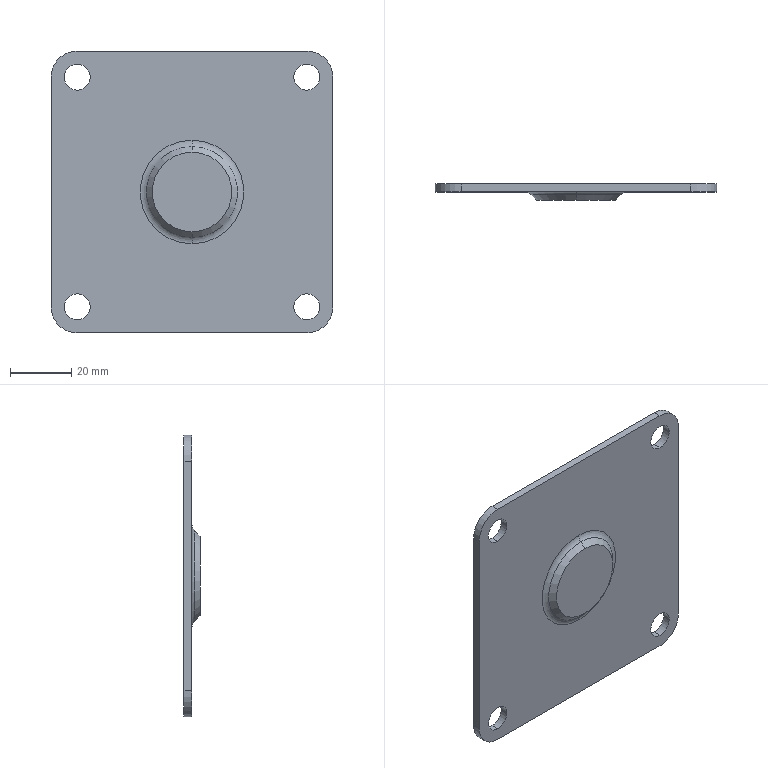Part | SolidWorks | features BaseBody 1 | 1 solid | 37 faces | box 92 x 5.3 x 92 mm | volume 22833 mm3 | cylinder 16 | torus 10 | plane 9 | cone 2 | commonest cylinder face diameters 8.5 x8 17 x6 20 x2
STEP:
#1=CARTESIAN_POINT('',(0.,0.,-13.));
#2=VERTEX_POINT('',#1);
#3=CARTESIAN_POINT('',(0.,0.,13.));
#4=VERTEX_POINT('',#3);
#5=CARTESIAN_POINT('',(0.,0.,0.));
#6=DIRECTION('',(0.,-1.,0.));
#7=DIRECTION('',(0.,0.,-1.));
#8=AXIS2_PLACEMENT_3D('',#5,#6,#7);
#9=CIRCLE('',#8,13.);
#10=EDGE_CURVE('',#2,#4,#9,.T.);
#11=ORIENTED_EDGE('',*,*,#10,.F.);
#12=CARTESIAN_POINT('',(0.,1.821,-14.821));
#13=VERTEX_POINT('',#12);
#14=CARTESIAN_POINT('',(0.,1.821,-14.821));
#15=DIRECTION('',(0.,0.7071,-0.7071));
#16=VECTOR('',#15,1000.);
#17=LINE('',#14,#16);
#18=EDGE_CURVE('',#2,#13,#17,.T.);
#19=ORIENTED_EDGE('',*,*,#18,.T.);
#20=CARTESIAN_POINT('',(0.,1.821,14.821));
#21=VERTEX_POINT('',#20);
#22=CARTESIAN_POINT('',(0.,1.821,0.));
#23=DIRECTION('',(0.,-1.,0.));
#24=DIRECTION('',(0.,0.,-1.));
#25=AXIS2_PLACEMENT_3D('',#22,#23,#24);
#26=CIRCLE('',#25,14.821);
#27=EDGE_CURVE('',#13,#21,#26,.T.);
#28=ORIENTED_EDGE('',*,*,#27,.T.);
#29=CARTESIAN_POINT('',(0.,1.821,14.821));
#30=DIRECTION('',(0.,0.7071,0.7071));
#31=VECTOR('',#30,1000.);
#32=LINE('',#29,#31);
#33=EDGE_CURVE('',#4,#21,#32,.T.);
#34=ORIENTED_EDGE('',*,*,#33,.F.);
#35=EDGE_LOOP('',(#11,#19,#28,#34));
#36=FACE_OUTER_BOUND('',#35,.T.);
#37=CARTESIAN_POINT('',(0.,1.821,0.));
#38=DIRECTION('',(0.,1.,0.));
#39=DIRECTION('',(0.,0.,1.));
#40=AXIS2_PLACEMENT_3D('',#37,#38,#39);
#41=CONICAL_SURFACE('',#40,14.821,0.7854);
#42=ADVANCED_FACE('',(#36),#41,.T.);
#43=CARTESIAN_POINT('',(0.,1.821,0.));
#44=DIRECTION('',(0.,-1.,0.));
#45=DIRECTION('',(0.,0.,-1.));
#46=AXIS2_PLACEMENT_3D('',#43,#44,#45);
#47=CIRCLE('',#46,14.821);
#48=EDGE_CURVE('',#21,#13,#47,.T.);
#49=ORIENTED_EDGE('',*,*,#48,.F.);
#50=CARTESIAN_POINT('',(0.,2.7,16.943));
#51=VERTEX_POINT('',#50);
#52=CARTESIAN_POINT('',(0.,-0.3,16.943));
#53=DIRECTION('',(1.,0.,0.));
#54=DIRECTION('',(0.,0.,-1.));
#55=AXIS2_PLACEMENT_3D('',#52,#53,#54);
#56=CIRCLE('',#55,3.);
#57=EDGE_CURVE('',#21,#51,#56,.T.);
#58=ORIENTED_EDGE('',*,*,#57,.T.);
#59=CARTESIAN_POINT('',(0.,2.7,-16.943));
#60=VERTEX_POINT('',#59);
#61=CARTESIAN_POINT('',(0.,2.7,0.));
#62=DIRECTION('',(0.,-1.,0.));
#63=DIRECTION('',(0.,0.,-1.));
#64=AXIS2_PLACEMENT_3D('',#61,#62,#63);
#65=CIRCLE('',#64,16.943);
#66=EDGE_CURVE('',#51,#60,#65,.T.);
#67=ORIENTED_EDGE('',*,*,#66,.T.);
#68=CARTESIAN_POINT('',(0.,-0.3,-16.943));
#69=DIRECTION('',(-1.,0.,0.));
#70=DIRECTION('',(0.,0.,1.));
#71=AXIS2_PLACEMENT_3D('',#68,#69,#70);
#72=CIRCLE('',#71,3.);
#73=EDGE_CURVE('',#13,#60,#72,.T.);
#74=ORIENTED_EDGE('',*,*,#73,.F.);
#75=EDGE_LOOP('',(#49,#58,#67,#74));
#76=FACE_OUTER_BOUND('',#75,.T.);
#77=CARTESIAN_POINT('',(0.,-0.3,0.));
#78=DIRECTION('',(0.,-1.,0.));
#79=DIRECTION('',(0.,0.,-1.));
#80=AXIS2_PLACEMENT_3D('',#77,#78,#79);
#81=TOROIDAL_SURFACE('',#80,16.943,3.);
#82=ADVANCED_FACE('',(#76),#81,.F.);
#83=CARTESIAN_POINT('',(-37.5,5.3,-41.75));
#84=VERTEX_POINT('',#83);
#85=CARTESIAN_POINT('',(-37.5,5.3,-33.25));
#86=VERTEX_POINT('',#85);
#87=CARTESIAN_POINT('',(-37.5,5.3,-37.5));
#88=DIRECTION('',(0.,1.,0.));
#89=DIRECTION('',(0.,0.,-1.));
#90=AXIS2_PLACEMENT_3D('',#87,#88,#89);
#91=CIRCLE('',#90,4.25);
#92=EDGE_CURVE('',#84,#86,#91,.T.);
#93=ORIENTED_EDGE('',*,*,#92,.T.);
#94=CARTESIAN_POINT('',(-37.5,2.7,-33.25));
#95=VERTEX_POINT('',#94);
#96=CARTESIAN_POINT('',(-37.5,5.6,-33.25));
#97=DIRECTION('',(0.,-1.,0.));
#98=VECTOR('',#97,1000.);
#99=LINE('',#96,#98);
#100=EDGE_CURVE('',#86,#95,#99,.T.);
#101=ORIENTED_EDGE('',*,*,#100,.T.);
#102=CARTESIAN_POINT('',(-37.5,2.7,-41.75));
#103=VERTEX_POINT('',#102);
#104=CARTESIAN_POINT('',(-37.5,2.7,-37.5));
#105=DIRECTION('',(0.,-1.,0.));
#106=DIRECTION('',(0.,0.,1.));
#107=AXIS2_PLACEMENT_3D('',#104,#105,#106);
#108=CIRCLE('',#107,4.25);
#109=EDGE_CURVE('',#95,#103,#108,.T.);
#110=ORIENTED_EDGE('',*,*,#109,.T.);
#111=CARTESIAN_POINT('',(-37.5,5.6,-41.75));
#112=DIRECTION('',(0.,-1.,0.));
#113=VECTOR('',#112,1000.);
#114=LINE('',#111,#113);
#115=EDGE_CURVE('',#84,#103,#114,.T.);
#116=ORIENTED_EDGE('',*,*,#115,.F.);
#117=EDGE_LOOP('',(#93,#101,#110,#116));
#118=FACE_OUTER_BOUND('',#117,.T.);
#119=CARTESIAN_POINT('',(-37.5,5.6,-37.5));
#120=DIRECTION('',(0.,-1.,0.));
#121=DIRECTION('',(0.,0.,-1.));
#122=AXIS2_PLACEMENT_3D('',#119,#120,#121);
#123=CYLINDRICAL_SURFACE('',#122,4.25);
#124=ADVANCED_FACE('',(#118),#123,.F.);
#125=CARTESIAN_POINT('',(-37.5,5.3,33.25));
#126=VERTEX_POINT('',#125);
#127=CARTESIAN_POINT('',(-37.5,5.3,41.75));
#128=VERTEX_POINT('',#127);
#129=CARTESIAN_POINT('',(-37.5,5.3,37.5));
#130=DIRECTION('',(0.,1.,0.));
#131=DIRECTION('',(0.,0.,-1.));
#132=AXIS2_PLACEMENT_3D('',#129,#130,#131);
#133=CIRCLE('',#132,4.25);
#134=EDGE_CURVE('',#126,#128,#133,.T.);
#135=ORIENTED_EDGE('',*,*,#134,.T.);
#136=CARTESIAN_POINT('',(-37.5,2.7,41.75));
#137=VERTEX_POINT('',#136);
#138=CARTESIAN_POINT('',(-37.5,5.6,41.75));
#139=DIRECTION('',(0.,-1.,0.));
#140=VECTOR('',#139,1000.);
#141=LINE('',#138,#140);
#142=EDGE_CURVE('',#128,#137,#141,.T.);
#143=ORIENTED_EDGE('',*,*,#142,.T.);
#144=CARTESIAN_POINT('',(-37.5,2.7,33.25));
#145=VERTEX_POINT('',#144);
#146=CARTESIAN_POINT('',(-37.5,2.7,37.5));
#147=DIRECTION('',(0.,-1.,0.));
#148=DIRECTION('',(0.,0.,1.));
#149=AXIS2_PLACEMENT_3D('',#146,#147,#148);
#150=CIRCLE('',#149,4.25);
#151=EDGE_CURVE('',#137,#145,#150,.T.);
#152=ORIENTED_EDGE('',*,*,#151,.T.);
#153=CARTESIAN_POINT('',(-37.5,5.6,33.25));
#154=DIRECTION('',(0.,-1.,0.));
#155=VECTOR('',#154,1000.);
#156=LINE('',#153,#155);
#157=EDGE_CURVE('',#126,#145,#156,.T.);
#158=ORIENTED_EDGE('',*,*,#157,.F.);
#159=EDGE_LOOP('',(#135,#143,#152,#158));
#160=FACE_OUTER_BOUND('',#159,.T.);
#161=CARTESIAN_POINT('',(-37.5,5.6,37.5));
#162=DIRECTION('',(0.,-1.,0.));
#163=DIRECTION('',(0.,0.,-1.));
#164=AXIS2_PLACEMENT_3D('',#161,#162,#163);
#165=CYLINDRICAL_SURFACE('',#164,4.25);
#166=ADVANCED_FACE('',(#160),#165,.F.);
#167=CARTESIAN_POINT('',(37.5,5.3,33.25));
#168=VERTEX_POINT('',#167);
#169=CARTESIAN_POINT('',(37.5,5.3,41.75));
#170=VERTEX_POINT('',#169);
#171=CARTESIAN_POINT('',(37.5,5.3,37.5));
#172=DIRECTION('',(0.,1.,0.));
#173=DIRECTION('',(0.,0.,-1.));
#174=AXIS2_PLACEMENT_3D('',#171,#172,#173);
#175=CIRCLE('',#174,4.25);
#176=EDGE_CURVE('',#168,#170,#175,.T.);
#177=ORIENTED_EDGE('',*,*,#176,.T.);
#178=CARTESIAN_POINT('',(37.5,2.7,41.75));
#179=VERTEX_POINT('',#178);
#180=CARTESIAN_POINT('',(37.5,5.6,41.75));
#181=DIRECTION('',(0.,-1.,0.));
#182=VECTOR('',#181,1000.);
#183=LINE('',#180,#182);
#184=EDGE_CURVE('',#170,#179,#183,.T.);
#185=ORIENTED_EDGE('',*,*,#184,.T.);
#186=CARTESIAN_POINT('',(37.5,2.7,33.25));
#187=VERTEX_POINT('',#186);
#188=CARTESIAN_POINT('',(37.5,2.7,37.5));
#189=DIRECTION('',(0.,-1.,0.));
#190=DIRECTION('',(0.,0.,1.));
#191=AXIS2_PLACEMENT_3D('',#188,#189,#190);
#192=CIRCLE('',#191,4.25);
#193=EDGE_CURVE('',#179,#187,#192,.T.);
#194=ORIENTED_EDGE('',*,*,#193,.T.);
#195=CARTESIAN_POINT('',(37.5,5.6,33.25));
#196=DIRECTION('',(0.,-1.,0.));
#197=VECTOR('',#196,1000.);
#198=LINE('',#195,#197);
#199=EDGE_CURVE('',#168,#187,#198,.T.);
#200=ORIENTED_EDGE('',*,*,#199,.F.);
#201=EDGE_LOOP('',(#177,#185,#194,#200));
#202=FACE_OUTER_BOUND('',#201,.T.);
#203=CARTESIAN_POINT('',(37.5,5.6,37.5));
#204=DIRECTION('',(0.,-1.,0.));
#205=DIRECTION('',(0.,0.,-1.));
#206=AXIS2_PLACEMENT_3D('',#203,#204,#205);
#207=CYLINDRICAL_SURFACE('',#206,4.25);
#208=ADVANCED_FACE('',(#202),#207,.F.);
#209=CARTESIAN_POINT('',(37.5,5.3,-41.75));
#210=VERTEX_POINT('',#209);
#211=CARTESIAN_POINT('',(37.5,5.3,-33.25));
#212=VERTEX_POINT('',#211);
#213=CARTESIAN_POINT('',(37.5,5.3,-37.5));
#214=DIRECTION('',(0.,1.,0.));
#215=DIRECTION('',(0.,0.,-1.));
#216=AXIS2_PLACEMENT_3D('',#213,#214,#215);
#217=CIRCLE('',#216,4.25);
#218=EDGE_CURVE('',#210,#212,#217,.T.);
#219=ORIENTED_EDGE('',*,*,#218,.T.);
#220=CARTESIAN_POINT('',(37.5,2.7,-33.25));
#221=VERTEX_POINT('',#220);
#222=CARTESIAN_POINT('',(37.5,5.6,-33.25));
#223=DIRECTION('',(0.,-1.,0.));
#224=VECTOR('',#223,1000.);
#225=LINE('',#222,#224);
#226=EDGE_CURVE('',#212,#221,#225,.T.);
#227=ORIENTED_EDGE('',*,*,#226,.T.);
#228=CARTESIAN_POINT('',(37.5,2.7,-41.75));
#229=VERTEX_POINT('',#228);
#230=CARTESIAN_POINT('',(37.5,2.7,-37.5));
#231=DIRECTION('',(0.,-1.,0.));
#232=DIRECTION('',(0.,0.,1.));
#233=AXIS2_PLACEMENT_3D('',#230,#231,#232);
#234=CIRCLE('',#233,4.25);
#235=EDGE_CURVE('',#221,#229,#234,.T.);
#236=ORIENTED_EDGE('',*,*,#235,.T.);
#237=CARTESIAN_POINT('',(37.5,5.6,-41.75));
#238=DIRECTION('',(0.,-1.,0.));
#239=VECTOR('',#238,1000.);
#240=LINE('',#237,#239);
#241=EDGE_CURVE('',#210,#229,#240,.T.);
#242=ORIENTED_EDGE('',*,*,#241,.F.);
#243=EDGE_LOOP('',(#219,#227,#236,#242));
#244=FACE_OUTER_BOUND('',#243,.T.);
#245=CARTESIAN_POINT('',(37.5,5.6,-37.5));
#246=DIRECTION('',(0.,-1.,0.));
#247=DIRECTION('',(0.,0.,-1.));
#248=AXIS2_PLACEMENT_3D('',#245,#246,#247);
#249=CYLINDRICAL_SURFACE('',#248,4.25);
#250=ADVANCED_FACE('',(#244),#249,.F.);
#251=CARTESIAN_POINT('',(0.,4.3,-10.));
#252=VERTEX_POINT('',#251);
#253=CARTESIAN_POINT('',(0.,4.3,10.));
#254=VERTEX_POINT('',#253);
#255=CARTESIAN_POINT('',(0.,4.3,0.));
#256=DIRECTION('',(0.,-1.,0.));
#257=DIRECTION('',(0.,0.,-1.));
#258=AXIS2_PLACEMENT_3D('',#255,#256,#257);
#259=CIRCLE('',#258,10.);
#260=EDGE_CURVE('',#252,#254,#259,.T.);
#261=ORIENTED_EDGE('',*,*,#260,.T.);
#262=CARTESIAN_POINT('',(0.,5.3,11.));
#263=VERTEX_POINT('',#262);
#264=CARTESIAN_POINT('',(0.,4.3,11.));
#265=DIRECTION('',(1.,0.,0.));
#266=DIRECTION('',(0.,0.,-1.));
#267=AXIS2_PLACEMENT_3D('',#264,#265,#266);
#268=CIRCLE('',#267,1.);
#269=EDGE_CURVE('',#254,#263,#268,.T.);
#270=ORIENTED_EDGE('',*,*,#269,.T.);
#271=CARTESIAN_POINT('',(0.,5.3,-11.));
#272=VERTEX_POINT('',#271);
#273=CARTESIAN_POINT('',(0.,5.3,0.));
#274=DIRECTION('',(0.,-1.,0.));
#275=DIRECTION('',(0.,0.,-1.));
#276=AXIS2_PLACEMENT_3D('',#273,#274,#275);
#277=CIRCLE('',#276,11.);
#278=EDGE_CURVE('',#272,#263,#277,.T.);
#279=ORIENTED_EDGE('',*,*,#278,.F.);
#280=CARTESIAN_POINT('',(0.,4.3,-11.));
#281=DIRECTION('',(-1.,0.,0.));
#282=DIRECTION('',(0.,0.,1.));
#283=AXIS2_PLACEMENT_3D('',#280,#281,#282);
#284=CIRCLE('',#283,1.);
#285=EDGE_CURVE('',#252,#272,#284,.T.);
#286=ORIENTED_EDGE('',*,*,#285,.F.);
#287=EDGE_LOOP('',(#261,#270,#279,#286));
#288=FACE_OUTER_BOUND('',#287,.T.);
#289=CARTESIAN_POINT('',(0.,4.3,0.));
#290=DIRECTION('',(0.,-1.,0.));
#291=DIRECTION('',(0.,0.,-1.));
#292=AXIS2_PLACEMENT_3D('',#289,#290,#291);
#293=TOROIDAL_SURFACE('',#292,11.,1.);
#294=ADVANCED_FACE('',(#288),#293,.T.);
#295=CARTESIAN_POINT('',(0.,4.3,0.));
#296=DIRECTION('',(0.,-1.,0.));
#297=DIRECTION('',(0.,0.,-1.));
#298=AXIS2_PLACEMENT_3D('',#295,#296,#297);
#299=CIRCLE('',#298,10.);
#300=EDGE_CURVE('',#254,#252,#299,.T.);
#301=ORIENTED_EDGE('',*,*,#300,.F.);
#302=CARTESIAN_POINT('',(0.,3.8,10.));
#303=VERTEX_POINT('',#302);
#304=CARTESIAN_POINT('',(0.,0.,10.));
#305=DIRECTION('',(0.,-1.,0.));
#306=VECTOR('',#305,1000.);
#307=LINE('',#304,#306);
#308=EDGE_CURVE('',#254,#303,#307,.T.);
#309=ORIENTED_EDGE('',*,*,#308,.T.);
#310=CARTESIAN_POINT('',(0.,3.8,-10.));
#311=VERTEX_POINT('',#310);
#312=CARTESIAN_POINT('',(0.,3.8,0.));
#313=DIRECTION('',(0.,-1.,0.));
#314=DIRECTION('',(0.,0.,-1.));
#315=AXIS2_PLACEMENT_3D('',#312,#313,#314);
#316=CIRCLE('',#315,10.);
#317=EDGE_CURVE('',#303,#311,#316,.T.);
#318=ORIENTED_EDGE('',*,*,#317,.T.);
#319=CARTESIAN_POINT('',(0.,0.,-10.));
#320=DIRECTION('',(0.,-1.,0.));
#321=VECTOR('',#320,1000.);
#322=LINE('',#319,#321);
#323=EDGE_CURVE('',#252,#311,#322,.T.);
#324=ORIENTED_EDGE('',*,*,#323,.F.);
#325=EDGE_LOOP('',(#301,#309,#318,#324));
#326=FACE_OUTER_BOUND('',#325,.T.);
#327=CARTESIAN_POINT('',(0.,0.,0.));
#328=DIRECTION('',(0.,-1.,0.));
#329=DIRECTION('',(0.,0.,-1.));
#330=AXIS2_PLACEMENT_3D('',#327,#328,#329);
#331=CYLINDRICAL_SURFACE('',#330,10.);
#332=ADVANCED_FACE('',(#326),#331,.F.);
#333=ORIENTED_EDGE('',*,*,#317,.F.);
#334=CARTESIAN_POINT('',(0.,3.3,9.5));
#335=VERTEX_POINT('',#334);
#336=CARTESIAN_POINT('',(0.,3.8,9.5));
#337=DIRECTION('',(1.,0.,0.));
#338=DIRECTION('',(0.,0.,-1.));
#339=AXIS2_PLACEMENT_3D('',#336,#337,#338);
#340=CIRCLE('',#339,0.5);
#341=EDGE_CURVE('',#303,#335,#340,.T.);
#342=ORIENTED_EDGE('',*,*,#341,.T.);
#343=CARTESIAN_POINT('',(0.,3.3,-9.5));
#344=VERTEX_POINT('',#343);
#345=CARTESIAN_POINT('',(0.,3.3,0.));
#346=DIRECTION('',(0.,-1.,0.));
#347=DIRECTION('',(0.,0.,-1.));
#348=AXIS2_PLACEMENT_3D('',#345,#346,#347);
#349=CIRCLE('',#348,9.5);
#350=EDGE_CURVE('',#335,#344,#349,.T.);
#351=ORIENTED_EDGE('',*,*,#350,.T.);
#352=CARTESIAN_POINT('',(0.,3.8,-9.5));
#353=DIRECTION('',(-1.,0.,0.));
#354=DIRECTION('',(0.,0.,1.));
#355=AXIS2_PLACEMENT_3D('',#352,#353,#354);
#356=CIRCLE('',#355,0.5);
#357=EDGE_CURVE('',#311,#344,#356,.T.);
#358=ORIENTED_EDGE('',*,*,#357,.F.);
#359=EDGE_LOOP('',(#333,#342,#351,#358));
#360=FACE_OUTER_BOUND('',#359,.T.);
#361=CARTESIAN_POINT('',(0.,3.8,0.));
#362=DIRECTION('',(0.,-1.,0.));
#363=DIRECTION('',(0.,0.,-1.));
#364=AXIS2_PLACEMENT_3D('',#361,#362,#363);
#365=TOROIDAL_SURFACE('',#364,9.5,0.5);
#366=ADVANCED_FACE('',(#360),#365,.F.);
#367=CARTESIAN_POINT('',(0.,3.3,9.));
#368=VERTEX_POINT('',#367);
#369=CARTESIAN_POINT('',(0.,3.3,-9.));
#370=VERTEX_POINT('',#369);
#371=CARTESIAN_POINT('',(0.,3.3,0.));
#372=DIRECTION('',(0.,-1.,0.));
#373=DIRECTION('',(0.,0.,-1.));
#374=AXIS2_PLACEMENT_3D('',#371,#372,#373);
#375=CIRCLE('',#374,9.);
#376=EDGE_CURVE('',#368,#370,#375,.T.);
#377=ORIENTED_EDGE('',*,*,#376,.F.);
#378=CARTESIAN_POINT('',(0.,3.8,8.5));
#379=VERTEX_POINT('',#378);
#380=CARTESIAN_POINT('',(0.,3.8,9.));
#381=DIRECTION('',(1.,0.,0.));
#382=DIRECTION('',(0.,0.,-1.));
#383=AXIS2_PLACEMENT_3D('',#380,#381,#382);
#384=CIRCLE('',#383,0.5);
#385=EDGE_CURVE('',#368,#379,#384,.T.);
#386=ORIENTED_EDGE('',*,*,#385,.T.);
#387=CARTESIAN_POINT('',(0.,3.8,-8.5));
#388=VERTEX_POINT('',#387);
#389=CARTESIAN_POINT('',(0.,3.8,0.));
#390=DIRECTION('',(0.,-1.,0.));
#391=DIRECTION('',(0.,0.,-1.));
#392=AXIS2_PLACEMENT_3D('',#389,#390,#391);
#393=CIRCLE('',#392,8.5);
#394=EDGE_CURVE('',#379,#388,#393,.T.);
#395=ORIENTED_EDGE('',*,*,#394,.T.);
#396=CARTESIAN_POINT('',(0.,3.8,-9.));
#397=DIRECTION('',(-1.,0.,0.));
#398=DIRECTION('',(0.,0.,1.));
#399=AXIS2_PLACEMENT_3D('',#396,#397,#398);
#400=CIRCLE('',#399,0.5);
#401=EDGE_CURVE('',#370,#388,#400,.T.);
#402=ORIENTED_EDGE('',*,*,#401,.F.);
#403=EDGE_LOOP('',(#377,#386,#395,#402));
#404=FACE_OUTER_BOUND('',#403,.T.);
#405=CARTESIAN_POINT('',(0.,3.8,0.));
#406=DIRECTION('',(0.,-1.,0.));
#407=DIRECTION('',(0.,0.,-1.));
#408=AXIS2_PLACEMENT_3D('',#405,#406,#407);
#409=TOROIDAL_SURFACE('',#408,9.,0.5);
#410=ADVANCED_FACE('',(#404),#409,.F.);
#411=CARTESIAN_POINT('',(0.,4.3,-8.5));
#412=VERTEX_POINT('',#411);
#413=CARTESIAN_POINT('',(0.,4.3,8.5));
#414=VERTEX_POINT('',#413);
#415=CARTESIAN_POINT('',(0.,4.3,0.));
#416=DIRECTION('',(0.,-1.,0.));
#417=DIRECTION('',(0.,0.,-1.));
#418=AXIS2_PLACEMENT_3D('',#415,#416,#417);
#419=CIRCLE('',#418,8.5);
#420=EDGE_CURVE('',#412,#414,#419,.T.);
#421=ORIENTED_EDGE('',*,*,#420,.T.);
#422=CARTESIAN_POINT('',(0.,0.,8.5));
#423=DIRECTION('',(0.,-1.,0.));
#424=VECTOR('',#423,1000.);
#425=LINE('',#422,#424);
#426=EDGE_CURVE('',#414,#379,#425,.T.);
#427=ORIENTED_EDGE('',*,*,#426,.T.);
#428=CARTESIAN_POINT('',(0.,3.8,0.));
#429=DIRECTION('',(0.,-1.,0.));
#430=DIRECTION('',(0.,0.,-1.));
#431=AXIS2_PLACEMENT_3D('',#428,#429,#430);
#432=CIRCLE('',#431,8.5);
#433=EDGE_CURVE('',#388,#379,#432,.T.);
#434=ORIENTED_EDGE('',*,*,#433,.F.);
#435=CARTESIAN_POINT('',(0.,0.,-8.5));
#436=DIRECTION('',(0.,-1.,0.));
#437=VECTOR('',#436,1000.);
#438=LINE('',#435,#437);
#439=EDGE_CURVE('',#412,#388,#438,.T.);
#440=ORIENTED_EDGE('',*,*,#439,.F.);
#441=EDGE_LOOP('',(#421,#427,#434,#440));
#442=FACE_OUTER_BOUND('',#441,.T.);
#443=CARTESIAN_POINT('',(0.,0.,0.));
#444=DIRECTION('',(0.,-1.,0.));
#445=DIRECTION('',(0.,0.,-1.));
#446=AXIS2_PLACEMENT_3D('',#443,#444,#445);
#447=CYLINDRICAL_SURFACE('',#446,8.5);
#448=ADVANCED_FACE('',(#442),#447,.T.);
#449=CARTESIAN_POINT('',(0.,5.3,-7.5));
#450=VERTEX_POINT('',#449);
#451=CARTESIAN_POINT('',(0.,5.3,7.5));
#452=VERTEX_POINT('',#451);
#453=CARTESIAN_POINT('',(0.,5.3,0.));
#454=DIRECTION('',(0.,-1.,0.));
#455=DIRECTION('',(0.,0.,-1.));
#456=AXIS2_PLACEMENT_3D('',#453,#454,#455);
#457=CIRCLE('',#456,7.5);
#458=EDGE_CURVE('',#450,#452,#457,.T.);
#459=ORIENTED_EDGE('',*,*,#458,.T.);
#460=CARTESIAN_POINT('',(0.,4.3,7.5));
#461=DIRECTION('',(1.,0.,0.));
#462=DIRECTION('',(0.,0.,-1.));
#463=AXIS2_PLACEMENT_3D('',#460,#461,#462);
#464=CIRCLE('',#463,1.);
#465=EDGE_CURVE('',#452,#414,#464,.T.);
#466=ORIENTED_EDGE('',*,*,#465,.T.);
#467=ORIENTED_EDGE('',*,*,#420,.F.);
#468=CARTESIAN_POINT('',(0.,4.3,-7.5));
#469=DIRECTION('',(-1.,0.,0.));
#470=DIRECTION('',(0.,0.,1.));
#471=AXIS2_PLACEMENT_3D('',#468,#469,#470);
#472=CIRCLE('',#471,1.);
#473=EDGE_CURVE('',#450,#412,#472,.T.);
#474=ORIENTED_EDGE('',*,*,#473,.F.);
#475=EDGE_LOOP('',(#459,#466,#467,#474));
#476=FACE_OUTER_BOUND('',#475,.T.);
#477=CARTESIAN_POINT('',(0.,4.3,0.));
#478=DIRECTION('',(0.,-1.,0.));
#479=DIRECTION('',(0.,0.,-1.));
#480=AXIS2_PLACEMENT_3D('',#477,#478,#479);
#481=TOROIDAL_SURFACE('',#480,7.5,1.);
#482=ADVANCED_FACE('',(#476),#481,.T.);
#483=ORIENTED_EDGE('',*,*,#458,.F.);
#484=CARTESIAN_POINT('',(0.,5.3,0.));
#485=DIRECTION('',(0.,-1.,0.));
#486=DIRECTION('',(0.,0.,-1.));
#487=AXIS2_PLACEMENT_3D('',#484,#485,#486);
#488=CIRCLE('',#487,7.5);
#489=EDGE_CURVE('',#452,#450,#488,.T.);
#490=ORIENTED_EDGE('',*,*,#489,.F.);
#491=EDGE_LOOP('',(#483,#490));
#492=FACE_OUTER_BOUND('',#491,.T.);
#493=CARTESIAN_POINT('',(0.,5.3,0.));
#494=DIRECTION('',(0.,-1.,0.));
#495=DIRECTION('',(0.,0.,-1.));
#496=AXIS2_PLACEMENT_3D('',#493,#494,#495);
#497=PLANE('',#496);
#498=ADVANCED_FACE('',(#492),#497,.F.);
#499=ORIENTED_EDGE('',*,*,#465,.F.);
#500=ORIENTED_EDGE('',*,*,#489,.T.);
#501=ORIENTED_EDGE('',*,*,#473,.T.);
#502=CARTESIAN_POINT('',(0.,4.3,0.));
#503=DIRECTION('',(0.,-1.,0.));
#504=DIRECTION('',(0.,0.,-1.));
#505=AXIS2_PLACEMENT_3D('',#502,#503,#504);
#506=CIRCLE('',#505,8.5);
#507=EDGE_CURVE('',#414,#412,#506,.T.);
#508=ORIENTED_EDGE('',*,*,#507,.F.);
#509=EDGE_LOOP('',(#499,#500,#501,#508));
#510=FACE_OUTER_BOUND('',#509,.T.);
#511=CARTESIAN_POINT('',(0.,4.3,0.));
#512=DIRECTION('',(0.,-1.,0.));
#513=DIRECTION('',(0.,0.,-1.));
#514=AXIS2_PLACEMENT_3D('',#511,#512,#513);
#515=TOROIDAL_SURFACE('',#514,7.5,1.);
#516=ADVANCED_FACE('',(#510),#515,.T.);
#517=ORIENTED_EDGE('',*,*,#426,.F.);
#518=ORIENTED_EDGE('',*,*,#507,.T.);
#519=ORIENTED_EDGE('',*,*,#439,.T.);
#520=ORIENTED_EDGE('',*,*,#394,.F.);
#521=EDGE_LOOP('',(#517,#518,#519,#520));
#522=FACE_OUTER_BOUND('',#521,.T.);
#523=CARTESIAN_POINT('',(0.,0.,0.));
#524=DIRECTION('',(0.,-1.,0.));
#525=DIRECTION('',(0.,0.,-1.));
#526=AXIS2_PLACEMENT_3D('',#523,#524,#525);
#527=CYLINDRICAL_SURFACE('',#526,8.5);
#528=ADVANCED_FACE('',(#522),#527,.T.);
#529=ORIENTED_EDGE('',*,*,#385,.F.);
#530=CARTESIAN_POINT('',(0.,3.3,0.));
#531=DIRECTION('',(0.,-1.,0.));
#532=DIRECTION('',(0.,0.,-1.));
#533=AXIS2_PLACEMENT_3D('',#530,#531,#532);
#534=CIRCLE('',#533,9.);
#535=EDGE_CURVE('',#370,#368,#534,.T.);
#536=ORIENTED_EDGE('',*,*,#535,.F.);
#537=ORIENTED_EDGE('',*,*,#401,.T.);
#538=ORIENTED_EDGE('',*,*,#433,.T.);
#539=EDGE_LOOP('',(#529,#536,#537,#538));
#540=FACE_OUTER_BOUND('',#539,.T.);
#541=CARTESIAN_POINT('',(0.,3.8,0.));
#542=DIRECTION('',(0.,-1.,0.));
#543=DIRECTION('',(0.,0.,-1.));
#544=AXIS2_PLACEMENT_3D('',#541,#542,#543);
#545=TOROIDAL_SURFACE('',#544,9.,0.5);
#546=ADVANCED_FACE('',(#540),#545,.F.);
#547=CARTESIAN_POINT('',(0.,3.3,0.));
#548=DIRECTION('',(0.,-1.,0.));
#549=DIRECTION('',(0.,0.,-1.));
#550=AXIS2_PLACEMENT_3D('',#547,#548,#549);
#551=CIRCLE('',#550,9.5);
#552=EDGE_CURVE('',#344,#335,#551,.T.);
#553=ORIENTED_EDGE('',*,*,#552,.F.);
#554=ORIENTED_EDGE('',*,*,#350,.F.);
#555=EDGE_LOOP('',(#553,#554));
#556=FACE_OUTER_BOUND('',#555,.T.);
#557=ORIENTED_EDGE('',*,*,#535,.T.);
#558=ORIENTED_EDGE('',*,*,#376,.T.);
#559=EDGE_LOOP('',(#557,#558));
#560=FACE_BOUND('',#559,.T.);
#561=CARTESIAN_POINT('',(9.,3.3,0.));
#562=DIRECTION('',(0.,-1.,0.));
#563=DIRECTION('',(0.,0.,-1.));
#564=AXIS2_PLACEMENT_3D('',#561,#562,#563);
#565=PLANE('',#564);
#566=ADVANCED_FACE('',(#556,#560),#565,.F.);
#567=ORIENTED_EDGE('',*,*,#341,.F.);
#568=CARTESIAN_POINT('',(0.,3.8,0.));
#569=DIRECTION('',(0.,-1.,0.));
#570=DIRECTION('',(0.,0.,-1.));
#571=AXIS2_PLACEMENT_3D('',#568,#569,#570);
#572=CIRCLE('',#571,10.);
#573=EDGE_CURVE('',#311,#303,#572,.T.);
#574=ORIENTED_EDGE('',*,*,#573,.F.);
#575=ORIENTED_EDGE('',*,*,#357,.T.);
#576=ORIENTED_EDGE('',*,*,#552,.T.);
#577=EDGE_LOOP('',(#567,#574,#575,#576));
#578=FACE_OUTER_BOUND('',#577,.T.);
#579=CARTESIAN_POINT('',(0.,3.8,0.));
#580=DIRECTION('',(0.,-1.,0.));
#581=DIRECTION('',(0.,0.,-1.));
#582=AXIS2_PLACEMENT_3D('',#579,#580,#581);
#583=TOROIDAL_SURFACE('',#582,9.5,0.5);
#584=ADVANCED_FACE('',(#578),#583,.F.);
#585=ORIENTED_EDGE('',*,*,#308,.F.);
#586=ORIENTED_EDGE('',*,*,#260,.F.);
#587=ORIENTED_EDGE('',*,*,#323,.T.);
#588=ORIENTED_EDGE('',*,*,#573,.T.);
#589=EDGE_LOOP('',(#585,#586,#587,#588));
#590=FACE_OUTER_BOUND('',#589,.T.);
#591=CARTESIAN_POINT('',(0.,0.,0.));
#592=DIRECTION('',(0.,-1.,0.));
#593=DIRECTION('',(0.,0.,-1.));
#594=AXIS2_PLACEMENT_3D('',#591,#592,#593);
#595=CYLINDRICAL_SURFACE('',#594,10.);
#596=ADVANCED_FACE('',(#590),#595,.F.);
#597=ORIENTED_EDGE('',*,*,#269,.F.);
#598=ORIENTED_EDGE('',*,*,#300,.T.);
#599=ORIENTED_EDGE('',*,*,#285,.T.);
#600=CARTESIAN_POINT('',(0.,5.3,0.));
#601=DIRECTION('',(0.,-1.,0.));
#602=DIRECTION('',(0.,0.,-1.));
#603=AXIS2_PLACEMENT_3D('',#600,#601,#602);
#604=CIRCLE('',#603,11.);
#605=EDGE_CURVE('',#263,#272,#604,.T.);
#606=ORIENTED_EDGE('',*,*,#605,.F.);
#607=EDGE_LOOP('',(#597,#598,#599,#606));
#608=FACE_OUTER_BOUND('',#607,.T.);
#609=CARTESIAN_POINT('',(0.,4.3,0.));
#610=DIRECTION('',(0.,-1.,0.));
#611=DIRECTION('',(0.,0.,-1.));
#612=AXIS2_PLACEMENT_3D('',#609,#610,#611);
#613=TOROIDAL_SURFACE('',#612,11.,1.);
#614=ADVANCED_FACE('',(#608),#613,.T.);
#615=CARTESIAN_POINT('',(46.,5.3,37.5));
#616=VERTEX_POINT('',#615);
#617=CARTESIAN_POINT('',(46.,5.3,-37.5));
#618=VERTEX_POINT('',#617);
#619=CARTESIAN_POINT('',(46.,5.3,37.5));
#620=DIRECTION('',(0.,0.,-1.));
#621=VECTOR('',#620,1000.);
#622=LINE('',#619,#621);
#623=EDGE_CURVE('',#616,#618,#622,.T.);
#624=ORIENTED_EDGE('',*,*,#623,.T.);
#625=CARTESIAN_POINT('',(37.5,5.3,-46.));
#626=VERTEX_POINT('',#625);
#627=CARTESIAN_POINT('',(37.5,5.3,-37.5));
#628=DIRECTION('',(0.,1.,0.));
#629=DIRECTION('',(1.,0.,0.));
#630=AXIS2_PLACEMENT_3D('',#627,#628,#629);
#631=CIRCLE('',#630,8.5);
#632=EDGE_CURVE('',#618,#626,#631,.T.);
#633=ORIENTED_EDGE('',*,*,#632,.T.);
#634=CARTESIAN_POINT('',(-37.5,5.3,-46.));
#635=VERTEX_POINT('',#634);
#636=CARTESIAN_POINT('',(37.5,5.3,-46.));
#637=DIRECTION('',(-1.,0.,0.));
#638=VECTOR('',#637,1000.);
#639=LINE('',#636,#638);
#640=EDGE_CURVE('',#626,#635,#639,.T.);
#641=ORIENTED_EDGE('',*,*,#640,.T.);
#642=CARTESIAN_POINT('',(-46.,5.3,-37.5));
#643=VERTEX_POINT('',#642);
#644=CARTESIAN_POINT('',(-37.5,5.3,-37.5));
#645=DIRECTION('',(0.,1.,0.));
#646=DIRECTION('',(0.,0.,-1.));
#647=AXIS2_PLACEMENT_3D('',#644,#645,#646);
#648=CIRCLE('',#647,8.5);
#649=EDGE_CURVE('',#635,#643,#648,.T.);
#650=ORIENTED_EDGE('',*,*,#649,.T.);
#651=CARTESIAN_POINT('',(-46.,5.3,37.5));
#652=VERTEX_POINT('',#651);
#653=CARTESIAN_POINT('',(-46.,5.3,-37.5));
#654=DIRECTION('',(0.,0.,1.));
#655=VECTOR('',#654,1000.);
#656=LINE('',#653,#655);
#657=EDGE_CURVE('',#643,#652,#656,.T.);
#658=ORIENTED_EDGE('',*,*,#657,.T.);
#659=CARTESIAN_POINT('',(-37.5,5.3,46.));
#660=VERTEX_POINT('',#659);
#661=CARTESIAN_POINT('',(-37.5,5.3,37.5));
#662=DIRECTION('',(0.,1.,0.));
#663=DIRECTION('',(-1.,0.,0.));
#664=AXIS2_PLACEMENT_3D('',#661,#662,#663);
#665=CIRCLE('',#664,8.5);
#666=EDGE_CURVE('',#652,#660,#665,.T.);
#667=ORIENTED_EDGE('',*,*,#666,.T.);
#668=CARTESIAN_POINT('',(37.5,5.3,46.));
#669=VERTEX_POINT('',#668);
#670=CARTESIAN_POINT('',(-37.5,5.3,46.));
#671=DIRECTION('',(1.,0.,0.));
#672=VECTOR('',#671,1000.);
#673=LINE('',#670,#672);
#674=EDGE_CURVE('',#660,#669,#673,.T.);
#675=ORIENTED_EDGE('',*,*,#674,.T.);
#676=CARTESIAN_POINT('',(37.5,5.3,37.5));
#677=DIRECTION('',(0.,1.,0.));
#678=DIRECTION('',(0.,0.,1.));
#679=AXIS2_PLACEMENT_3D('',#676,#677,#678);
#680=CIRCLE('',#679,8.5);
#681=EDGE_CURVE('',#669,#616,#680,.T.);
#682=ORIENTED_EDGE('',*,*,#681,.T.);
#683=EDGE_LOOP('',(#624,#633,#641,#650,#658,#667,#675,#682));
#684=FACE_OUTER_BOUND('',#683,.T.);
#685=ORIENTED_EDGE('',*,*,#218,.F.);
#686=CARTESIAN_POINT('',(37.5,5.3,-37.5));
#687=DIRECTION('',(0.,1.,0.));
#688=DIRECTION('',(0.,0.,-1.));
#689=AXIS2_PLACEMENT_3D('',#686,#687,#688);
#690=CIRCLE('',#689,4.25);
#691=EDGE_CURVE('',#212,#210,#690,.T.);
#692=ORIENTED_EDGE('',*,*,#691,.F.);
#693=EDGE_LOOP('',(#685,#692));
#694=FACE_BOUND('',#693,.T.);
#695=ORIENTED_EDGE('',*,*,#176,.F.);
#696=CARTESIAN_POINT('',(37.5,5.3,37.5));
#697=DIRECTION('',(0.,1.,0.));
#698=DIRECTION('',(0.,0.,-1.));
#699=AXIS2_PLACEMENT_3D('',#696,#697,#698);
#700=CIRCLE('',#699,4.25);
#701=EDGE_CURVE('',#170,#168,#700,.T.);
#702=ORIENTED_EDGE('',*,*,#701,.F.);
#703=EDGE_LOOP('',(#695,#702));
#704=FACE_BOUND('',#703,.T.);
#705=ORIENTED_EDGE('',*,*,#134,.F.);
#706=CARTESIAN_POINT('',(-37.5,5.3,37.5));
#707=DIRECTION('',(0.,1.,0.));
#708=DIRECTION('',(0.,0.,-1.));
#709=AXIS2_PLACEMENT_3D('',#706,#707,#708);
#710=CIRCLE('',#709,4.25);
#711=EDGE_CURVE('',#128,#126,#710,.T.);
#712=ORIENTED_EDGE('',*,*,#711,.F.);
#713=EDGE_LOOP('',(#705,#712));
#714=FACE_BOUND('',#713,.T.);
#715=ORIENTED_EDGE('',*,*,#92,.F.);
#716=CARTESIAN_POINT('',(-37.5,5.3,-37.5));
#717=DIRECTION('',(0.,1.,0.));
#718=DIRECTION('',(0.,0.,-1.));
#719=AXIS2_PLACEMENT_3D('',#716,#717,#718);
#720=CIRCLE('',#719,4.25);
#721=EDGE_CURVE('',#86,#84,#720,.T.);
#722=ORIENTED_EDGE('',*,*,#721,.F.);
#723=EDGE_LOOP('',(#715,#722));
#724=FACE_BOUND('',#723,.T.);
#725=ORIENTED_EDGE('',*,*,#278,.T.);
#726=ORIENTED_EDGE('',*,*,#605,.T.);
#727=EDGE_LOOP('',(#725,#726));
#728=FACE_BOUND('',#727,.T.);
#729=CARTESIAN_POINT('',(11.,5.3,0.));
#730=DIRECTION('',(0.,-1.,0.));
#731=DIRECTION('',(0.,0.,-1.));
#732=AXIS2_PLACEMENT_3D('',#729,#730,#731);
#733=PLANE('',#732);
#734=ADVANCED_FACE('',(#684,#694,#704,#714,#724,#728),#733,.F.);
#735=CARTESIAN_POINT('',(46.,2.7,37.5));
#736=VERTEX_POINT('',#735);
#737=CARTESIAN_POINT('',(46.,5.3,37.5));
#738=DIRECTION('',(0.,-1.,0.));
#739=VECTOR('',#738,1000.);
#740=LINE('',#737,#739);
#741=EDGE_CURVE('',#616,#736,#740,.T.);
#742=ORIENTED_EDGE('',*,*,#741,.T.);
#743=CARTESIAN_POINT('',(46.,2.7,-37.5));
#744=VERTEX_POINT('',#743);
#745=CARTESIAN_POINT('',(46.,2.7,-37.5));
#746=DIRECTION('',(0.,0.,1.));
#747=VECTOR('',#746,1000.);
#748=LINE('',#745,#747);
#749=EDGE_CURVE('',#744,#736,#748,.T.);
#750=ORIENTED_EDGE('',*,*,#749,.F.);
#751=CARTESIAN_POINT('',(46.,5.3,-37.5));
#752=DIRECTION('',(0.,-1.,0.));
#753=VECTOR('',#752,1000.);
#754=LINE('',#751,#753);
#755=EDGE_CURVE('',#618,#744,#754,.T.);
#756=ORIENTED_EDGE('',*,*,#755,.F.);
#757=ORIENTED_EDGE('',*,*,#623,.F.);
#758=EDGE_LOOP('',(#742,#750,#756,#757));
#759=FACE_OUTER_BOUND('',#758,.T.);
#760=CARTESIAN_POINT('',(46.,5.6,37.5));
#761=DIRECTION('',(-1.,0.,0.));
#762=DIRECTION('',(0.,0.,1.));
#763=AXIS2_PLACEMENT_3D('',#760,#761,#762);
#764=PLANE('',#763);
#765=ADVANCED_FACE('',(#759),#764,.F.);
#766=ORIENTED_EDGE('',*,*,#755,.T.);
#767=CARTESIAN_POINT('',(37.5,2.7,-46.));
#768=VERTEX_POINT('',#767);
#769=CARTESIAN_POINT('',(37.5,2.7,-37.5));
#770=DIRECTION('',(0.,-1.,0.));
#771=DIRECTION('',(0.,0.,-1.));
#772=AXIS2_PLACEMENT_3D('',#769,#770,#771);
#773=CIRCLE('',#772,8.5);
#774=EDGE_CURVE('',#768,#744,#773,.T.);
#775=ORIENTED_EDGE('',*,*,#774,.F.);
#776=CARTESIAN_POINT('',(37.5,5.3,-46.));
#777=DIRECTION('',(0.,-1.,0.));
#778=VECTOR('',#777,1000.);
#779=LINE('',#776,#778);
#780=EDGE_CURVE('',#626,#768,#779,.T.);
#781=ORIENTED_EDGE('',*,*,#780,.F.);
#782=ORIENTED_EDGE('',*,*,#632,.F.);
#783=EDGE_LOOP('',(#766,#775,#781,#782));
#784=FACE_OUTER_BOUND('',#783,.T.);
#785=CARTESIAN_POINT('',(37.5,5.6,-37.5));
#786=DIRECTION('',(0.,-1.,0.));
#787=DIRECTION('',(0.,0.,-1.));
#788=AXIS2_PLACEMENT_3D('',#785,#786,#787);
#789=CYLINDRICAL_SURFACE('',#788,8.5);
#790=ADVANCED_FACE('',(#784),#789,.T.);
#791=ORIENTED_EDGE('',*,*,#780,.T.);
#792=CARTESIAN_POINT('',(-37.5,2.7,-46.));
#793=VERTEX_POINT('',#792);
#794=CARTESIAN_POINT('',(-37.5,2.7,-46.));
#795=DIRECTION('',(1.,0.,0.));
#796=VECTOR('',#795,1000.);
#797=LINE('',#794,#796);
#798=EDGE_CURVE('',#793,#768,#797,.T.);
#799=ORIENTED_EDGE('',*,*,#798,.F.);
#800=CARTESIAN_POINT('',(-37.5,5.3,-46.));
#801=DIRECTION('',(0.,-1.,0.));
#802=VECTOR('',#801,1000.);
#803=LINE('',#800,#802);
#804=EDGE_CURVE('',#635,#793,#803,.T.);
#805=ORIENTED_EDGE('',*,*,#804,.F.);
#806=ORIENTED_EDGE('',*,*,#640,.F.);
#807=EDGE_LOOP('',(#791,#799,#805,#806));
#808=FACE_OUTER_BOUND('',#807,.T.);
#809=CARTESIAN_POINT('',(37.5,5.6,-46.));
#810=DIRECTION('',(0.,0.,1.));
#811=DIRECTION('',(1.,0.,0.));
#812=AXIS2_PLACEMENT_3D('',#809,#810,#811);
#813=PLANE('',#812);
#814=ADVANCED_FACE('',(#808),#813,.F.);
#815=ORIENTED_EDGE('',*,*,#804,.T.);
#816=CARTESIAN_POINT('',(-46.,2.7,-37.5));
#817=VERTEX_POINT('',#816);
#818=CARTESIAN_POINT('',(-37.5,2.7,-37.5));
#819=DIRECTION('',(0.,-1.,0.));
#820=DIRECTION('',(-1.,0.,0.));
#821=AXIS2_PLACEMENT_3D('',#818,#819,#820);
#822=CIRCLE('',#821,8.5);
#823=EDGE_CURVE('',#817,#793,#822,.T.);
#824=ORIENTED_EDGE('',*,*,#823,.F.);
#825=CARTESIAN_POINT('',(-46.,5.3,-37.5));
#826=DIRECTION('',(0.,-1.,0.));
#827=VECTOR('',#826,1000.);
#828=LINE('',#825,#827);
#829=EDGE_CURVE('',#643,#817,#828,.T.);
#830=ORIENTED_EDGE('',*,*,#829,.F.);
#831=ORIENTED_EDGE('',*,*,#649,.F.);
#832=EDGE_LOOP('',(#815,#824,#830,#831));
#833=FACE_OUTER_BOUND('',#832,.T.);
#834=CARTESIAN_POINT('',(-37.5,5.6,-37.5));
#835=DIRECTION('',(0.,-1.,0.));
#836=DIRECTION('',(0.,0.,-1.));
#837=AXIS2_PLACEMENT_3D('',#834,#835,#836);
#838=CYLINDRICAL_SURFACE('',#837,8.5);
#839=ADVANCED_FACE('',(#833),#838,.T.);
#840=ORIENTED_EDGE('',*,*,#829,.T.);
#841=CARTESIAN_POINT('',(-46.,2.7,37.5));
#842=VERTEX_POINT('',#841);
#843=CARTESIAN_POINT('',(-46.,2.7,37.5));
#844=DIRECTION('',(0.,0.,-1.));
#845=VECTOR('',#844,1000.);
#846=LINE('',#843,#845);
#847=EDGE_CURVE('',#842,#817,#846,.T.);
#848=ORIENTED_EDGE('',*,*,#847,.F.);
#849=CARTESIAN_POINT('',(-46.,5.3,37.5));
#850=DIRECTION('',(0.,-1.,0.));
#851=VECTOR('',#850,1000.);
#852=LINE('',#849,#851);
#853=EDGE_CURVE('',#652,#842,#852,.T.);
#854=ORIENTED_EDGE('',*,*,#853,.F.);
#855=ORIENTED_EDGE('',*,*,#657,.F.);
#856=EDGE_LOOP('',(#840,#848,#854,#855));
#857=FACE_OUTER_BOUND('',#856,.T.);
#858=CARTESIAN_POINT('',(-46.,5.6,-37.5));
#859=DIRECTION('',(1.,0.,0.));
#860=DIRECTION('',(0.,0.,-1.));
#861=AXIS2_PLACEMENT_3D('',#858,#859,#860);
#862=PLANE('',#861);
#863=ADVANCED_FACE('',(#857),#862,.F.);
#864=ORIENTED_EDGE('',*,*,#853,.T.);
#865=CARTESIAN_POINT('',(-37.5,2.7,46.));
#866=VERTEX_POINT('',#865);
#867=CARTESIAN_POINT('',(-37.5,2.7,37.5));
#868=DIRECTION('',(0.,-1.,0.));
#869=DIRECTION('',(0.,0.,1.));
#870=AXIS2_PLACEMENT_3D('',#867,#868,#869);
#871=CIRCLE('',#870,8.5);
#872=EDGE_CURVE('',#866,#842,#871,.T.);
#873=ORIENTED_EDGE('',*,*,#872,.F.);
#874=CARTESIAN_POINT('',(-37.5,5.3,46.));
#875=DIRECTION('',(0.,-1.,0.));
#876=VECTOR('',#875,1000.);
#877=LINE('',#874,#876);
#878=EDGE_CURVE('',#660,#866,#877,.T.);
#879=ORIENTED_EDGE('',*,*,#878,.F.);
#880=ORIENTED_EDGE('',*,*,#666,.F.);
#881=EDGE_LOOP('',(#864,#873,#879,#880));
#882=FACE_OUTER_BOUND('',#881,.T.);
#883=CARTESIAN_POINT('',(-37.5,5.6,37.5));
#884=DIRECTION('',(0.,-1.,0.));
#885=DIRECTION('',(0.,0.,-1.));
#886=AXIS2_PLACEMENT_3D('',#883,#884,#885);
#887=CYLINDRICAL_SURFACE('',#886,8.5);
#888=ADVANCED_FACE('',(#882),#887,.T.);
#889=ORIENTED_EDGE('',*,*,#878,.T.);
#890=CARTESIAN_POINT('',(37.5,2.7,46.));
#891=VERTEX_POINT('',#890);
#892=CARTESIAN_POINT('',(37.5,2.7,46.));
#893=DIRECTION('',(-1.,0.,0.));
#894=VECTOR('',#893,1000.);
#895=LINE('',#892,#894);
#896=EDGE_CURVE('',#891,#866,#895,.T.);
#897=ORIENTED_EDGE('',*,*,#896,.F.);
#898=CARTESIAN_POINT('',(37.5,5.3,46.));
#899=DIRECTION('',(0.,-1.,0.));
#900=VECTOR('',#899,1000.);
#901=LINE('',#898,#900);
#902=EDGE_CURVE('',#669,#891,#901,.T.);
#903=ORIENTED_EDGE('',*,*,#902,.F.);
#904=ORIENTED_EDGE('',*,*,#674,.F.);
#905=EDGE_LOOP('',(#889,#897,#903,#904));
#906=FACE_OUTER_BOUND('',#905,.T.);
#907=CARTESIAN_POINT('',(-37.5,5.6,46.));
#908=DIRECTION('',(0.,0.,-1.));
#909=DIRECTION('',(-1.,0.,0.));
#910=AXIS2_PLACEMENT_3D('',#907,#908,#909);
#911=PLANE('',#910);
#912=ADVANCED_FACE('',(#906),#911,.F.);
#913=ORIENTED_EDGE('',*,*,#902,.T.);
#914=CARTESIAN_POINT('',(37.5,2.7,37.5));
#915=DIRECTION('',(0.,-1.,0.));
#916=DIRECTION('',(1.,0.,0.));
#917=AXIS2_PLACEMENT_3D('',#914,#915,#916);
#918=CIRCLE('',#917,8.5);
#919=EDGE_CURVE('',#736,#891,#918,.T.);
#920=ORIENTED_EDGE('',*,*,#919,.F.);
#921=ORIENTED_EDGE('',*,*,#741,.F.);
#922=ORIENTED_EDGE('',*,*,#681,.F.);
#923=EDGE_LOOP('',(#913,#920,#921,#922));
#924=FACE_OUTER_BOUND('',#923,.T.);
#925=CARTESIAN_POINT('',(37.5,5.6,37.5));
#926=DIRECTION('',(0.,-1.,0.));
#927=DIRECTION('',(0.,0.,-1.));
#928=AXIS2_PLACEMENT_3D('',#925,#926,#927);
#929=CYLINDRICAL_SURFACE('',#928,8.5);
#930=ADVANCED_FACE('',(#924),#929,.T.);
#931=ORIENTED_EDGE('',*,*,#226,.F.);
#932=ORIENTED_EDGE('',*,*,#691,.T.);
#933=ORIENTED_EDGE('',*,*,#241,.T.);
#934=CARTESIAN_POINT('',(37.5,2.7,-37.5));
#935=DIRECTION('',(0.,-1.,0.));
#936=DIRECTION('',(0.,0.,1.));
#937=AXIS2_PLACEMENT_3D('',#934,#935,#936);
#938=CIRCLE('',#937,4.25);
#939=EDGE_CURVE('',#229,#221,#938,.T.);
#940=ORIENTED_EDGE('',*,*,#939,.T.);
#941=EDGE_LOOP('',(#931,#932,#933,#940));
#942=FACE_OUTER_BOUND('',#941,.T.);
#943=CARTESIAN_POINT('',(37.5,5.6,-37.5));
#944=DIRECTION('',(0.,-1.,0.));
#945=DIRECTION('',(0.,0.,-1.));
#946=AXIS2_PLACEMENT_3D('',#943,#944,#945);
#947=CYLINDRICAL_SURFACE('',#946,4.25);
#948=ADVANCED_FACE('',(#942),#947,.F.);
#949=ORIENTED_EDGE('',*,*,#184,.F.);
#950=ORIENTED_EDGE('',*,*,#701,.T.);
#951=ORIENTED_EDGE('',*,*,#199,.T.);
#952=CARTESIAN_POINT('',(37.5,2.7,37.5));
#953=DIRECTION('',(0.,-1.,0.));
#954=DIRECTION('',(0.,0.,1.));
#955=AXIS2_PLACEMENT_3D('',#952,#953,#954);
#956=CIRCLE('',#955,4.25);
#957=EDGE_CURVE('',#187,#179,#956,.T.);
#958=ORIENTED_EDGE('',*,*,#957,.T.);
#959=EDGE_LOOP('',(#949,#950,#951,#958));
#960=FACE_OUTER_BOUND('',#959,.T.);
#961=CARTESIAN_POINT('',(37.5,5.6,37.5));
#962=DIRECTION('',(0.,-1.,0.));
#963=DIRECTION('',(0.,0.,-1.));
#964=AXIS2_PLACEMENT_3D('',#961,#962,#963);
#965=CYLINDRICAL_SURFACE('',#964,4.25);
#966=ADVANCED_FACE('',(#960),#965,.F.);
#967=ORIENTED_EDGE('',*,*,#142,.F.);
#968=ORIENTED_EDGE('',*,*,#711,.T.);
#969=ORIENTED_EDGE('',*,*,#157,.T.);
#970=CARTESIAN_POINT('',(-37.5,2.7,37.5));
#971=DIRECTION('',(0.,-1.,0.));
#972=DIRECTION('',(0.,0.,1.));
#973=AXIS2_PLACEMENT_3D('',#970,#971,#972);
#974=CIRCLE('',#973,4.25);
#975=EDGE_CURVE('',#145,#137,#974,.T.);
#976=ORIENTED_EDGE('',*,*,#975,.T.);
#977=EDGE_LOOP('',(#967,#968,#969,#976));
#978=FACE_OUTER_BOUND('',#977,.T.);
#979=CARTESIAN_POINT('',(-37.5,5.6,37.5));
#980=DIRECTION('',(0.,-1.,0.));
#981=DIRECTION('',(0.,0.,-1.));
#982=AXIS2_PLACEMENT_3D('',#979,#980,#981);
#983=CYLINDRICAL_SURFACE('',#982,4.25);
#984=ADVANCED_FACE('',(#978),#983,.F.);
#985=ORIENTED_EDGE('',*,*,#100,.F.);
#986=ORIENTED_EDGE('',*,*,#721,.T.);
#987=ORIENTED_EDGE('',*,*,#115,.T.);
#988=CARTESIAN_POINT('',(-37.5,2.7,-37.5));
#989=DIRECTION('',(0.,-1.,0.));
#990=DIRECTION('',(0.,0.,1.));
#991=AXIS2_PLACEMENT_3D('',#988,#989,#990);
#992=CIRCLE('',#991,4.25);
#993=EDGE_CURVE('',#103,#95,#992,.T.);
#994=ORIENTED_EDGE('',*,*,#993,.T.);
#995=EDGE_LOOP('',(#985,#986,#987,#994));
#996=FACE_OUTER_BOUND('',#995,.T.);
#997=CARTESIAN_POINT('',(-37.5,5.6,-37.5));
#998=DIRECTION('',(0.,-1.,0.));
#999=DIRECTION('',(0.,0.,-1.));
#1000=AXIS2_PLACEMENT_3D('',#997,#998,#999);
#1001=CYLINDRICAL_SURFACE('',#1000,4.25);
#1002=ADVANCED_FACE('',(#996),#1001,.F.);
#1003=CARTESIAN_POINT('',(0.,2.7,0.));
#1004=DIRECTION('',(0.,-1.,0.));
#1005=DIRECTION('',(0.,0.,-1.));
#1006=AXIS2_PLACEMENT_3D('',#1003,#1004,#1005);
#1007=CIRCLE('',#1006,16.943);
#1008=EDGE_CURVE('',#60,#51,#1007,.T.);
#1009=ORIENTED_EDGE('',*,*,#1008,.F.);
#1010=ORIENTED_EDGE('',*,*,#66,.F.);
#1011=EDGE_LOOP('',(#1009,#1010));
#1012=FACE_BOUND('',#1011,.T.);
#1013=ORIENTED_EDGE('',*,*,#939,.F.);
#1014=ORIENTED_EDGE('',*,*,#235,.F.);
#1015=EDGE_LOOP('',(#1013,#1014));
#1016=FACE_BOUND('',#1015,.T.);
#1017=ORIENTED_EDGE('',*,*,#957,.F.);
#1018=ORIENTED_EDGE('',*,*,#193,.F.);
#1019=EDGE_LOOP('',(#1017,#1018));
#1020=FACE_BOUND('',#1019,.T.);
#1021=ORIENTED_EDGE('',*,*,#975,.F.);
#1022=ORIENTED_EDGE('',*,*,#151,.F.);
#1023=EDGE_LOOP('',(#1021,#1022));
#1024=FACE_BOUND('',#1023,.T.);
#1025=ORIENTED_EDGE('',*,*,#993,.F.);
#1026=ORIENTED_EDGE('',*,*,#109,.F.);
#1027=EDGE_LOOP('',(#1025,#1026));
#1028=FACE_BOUND('',#1027,.T.);
#1029=ORIENTED_EDGE('',*,*,#847,.T.);
#1030=ORIENTED_EDGE('',*,*,#823,.T.);
#1031=ORIENTED_EDGE('',*,*,#798,.T.);
#1032=ORIENTED_EDGE('',*,*,#774,.T.);
#1033=ORIENTED_EDGE('',*,*,#749,.T.);
#1034=ORIENTED_EDGE('',*,*,#919,.T.);
#1035=ORIENTED_EDGE('',*,*,#896,.T.);
#1036=ORIENTED_EDGE('',*,*,#872,.T.);
#1037=EDGE_LOOP('',(#1029,#1030,#1031,#1032,#1033,#1034,#1035,#1036));
#1038=FACE_OUTER_BOUND('',#1037,.T.);
#1039=CARTESIAN_POINT('',(92.,2.7,0.));
#1040=DIRECTION('',(0.,1.,0.));
#1041=DIRECTION('',(0.,0.,1.));
#1042=AXIS2_PLACEMENT_3D('',#1039,#1040,#1041);
#1043=PLANE('',#1042);
#1044=ADVANCED_FACE('',(#1012,#1016,#1020,#1024,#1028,#1038),#1043,.F.);
#1045=ORIENTED_EDGE('',*,*,#57,.F.);
#1046=ORIENTED_EDGE('',*,*,#27,.F.);
#1047=ORIENTED_EDGE('',*,*,#73,.T.);
#1048=ORIENTED_EDGE('',*,*,#1008,.T.);
#1049=EDGE_LOOP('',(#1045,#1046,#1047,#1048));
#1050=FACE_OUTER_BOUND('',#1049,.T.);
#1051=CARTESIAN_POINT('',(0.,-0.3,0.));
#1052=DIRECTION('',(0.,-1.,0.));
#1053=DIRECTION('',(0.,0.,-1.));
#1054=AXIS2_PLACEMENT_3D('',#1051,#1052,#1053);
#1055=TOROIDAL_SURFACE('',#1054,16.943,3.);
#1056=ADVANCED_FACE('',(#1050),#1055,.F.);
#1057=ORIENTED_EDGE('',*,*,#18,.F.);
#1058=CARTESIAN_POINT('',(0.,0.,0.));
#1059=DIRECTION('',(0.,-1.,0.));
#1060=DIRECTION('',(0.,0.,-1.));
#1061=AXIS2_PLACEMENT_3D('',#1058,#1059,#1060);
#1062=CIRCLE('',#1061,13.);
#1063=EDGE_CURVE('',#4,#2,#1062,.T.);
#1064=ORIENTED_EDGE('',*,*,#1063,.F.);
#1065=ORIENTED_EDGE('',*,*,#33,.T.);
#1066=ORIENTED_EDGE('',*,*,#48,.T.);
#1067=EDGE_LOOP('',(#1057,#1064,#1065,#1066));
#1068=FACE_OUTER_BOUND('',#1067,.T.);
#1069=CARTESIAN_POINT('',(0.,1.821,0.));
#1070=DIRECTION('',(0.,1.,0.));
#1071=DIRECTION('',(0.,0.,1.));
#1072=AXIS2_PLACEMENT_3D('',#1069,#1070,#1071);
#1073=CONICAL_SURFACE('',#1072,14.821,0.7854);
#1074=ADVANCED_FACE('',(#1068),#1073,.T.);
#1075=ORIENTED_EDGE('',*,*,#1063,.T.);
#1076=ORIENTED_EDGE('',*,*,#10,.T.);
#1077=EDGE_LOOP('',(#1075,#1076));
#1078=FACE_OUTER_BOUND('',#1077,.T.);
#1079=CARTESIAN_POINT('',(13.,0.,0.));
#1080=DIRECTION('',(0.,1.,0.));
#1081=DIRECTION('',(0.,0.,1.));
#1082=AXIS2_PLACEMENT_3D('',#1079,#1080,#1081);
#1083=PLANE('',#1082);
#1084=ADVANCED_FACE('',(#1078),#1083,.F.);
#1085=CLOSED_SHELL('',(#42,#82,#124,#166,#208,#250,#294,#332,#366,#410,#448,#482,#498,#516,#528,#546,#566,#584,#596,#614,#734,#765,#790,#814,#839,#863,#888,#912,#930,#948,#966,#984,#1002,#1044,#1056,#1074,#1084));
#1086=MANIFOLD_SOLID_BREP('',#1085);
#1087=CARTESIAN_POINT('',(0.,0.,0.));
#1088=DIRECTION('',(0.,0.,1.));
#1089=DIRECTION('',(1.,0.,0.));
#1090=AXIS2_PLACEMENT_3D('',#1087,#1088,#1089);
#1091=(LENGTH_UNIT()NAMED_UNIT(*)SI_UNIT(.MILLI.,.METRE.));
#1092=UNCERTAINTY_MEASURE_WITH_UNIT(LENGTH_MEASURE(0.00001),#1091,'','');
#1093=(NAMED_UNIT(*)PLANE_ANGLE_UNIT()SI_UNIT($,.RADIAN.));
#1094=(NAMED_UNIT(*)SI_UNIT($,.STERADIAN.)SOLID_ANGLE_UNIT());
#1095=(GEOMETRIC_REPRESENTATION_CONTEXT(3)GLOBAL_UNCERTAINTY_ASSIGNED_CONTEXT((#1092))GLOBAL_UNIT_ASSIGNED_CONTEXT((#1091,#1093,#1094))REPRESENTATION_CONTEXT('',''));
#1096=ADVANCED_BREP_SHAPE_REPRESENTATION('',(#1086,#1090),#1095);